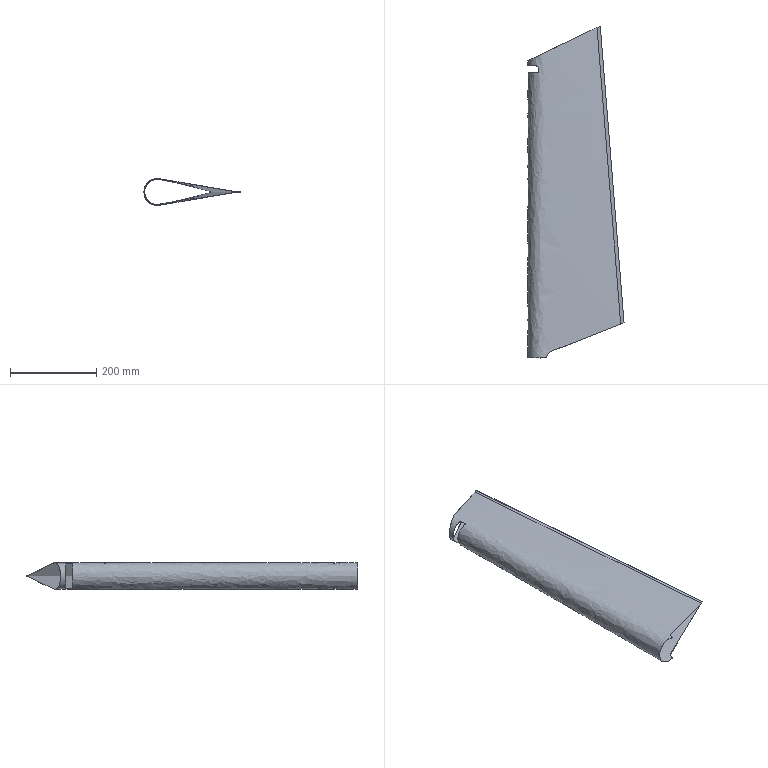Part | SolidWorks | features BaseBody 1 | 1 solid | 20 faces | box 222.493 x 768.769 x 62.001 mm | volume 74782 mm3 | plane 13 | cylinder 4 | spline 3 | commonest cylinder face diameters 12 x2 31.944 x2